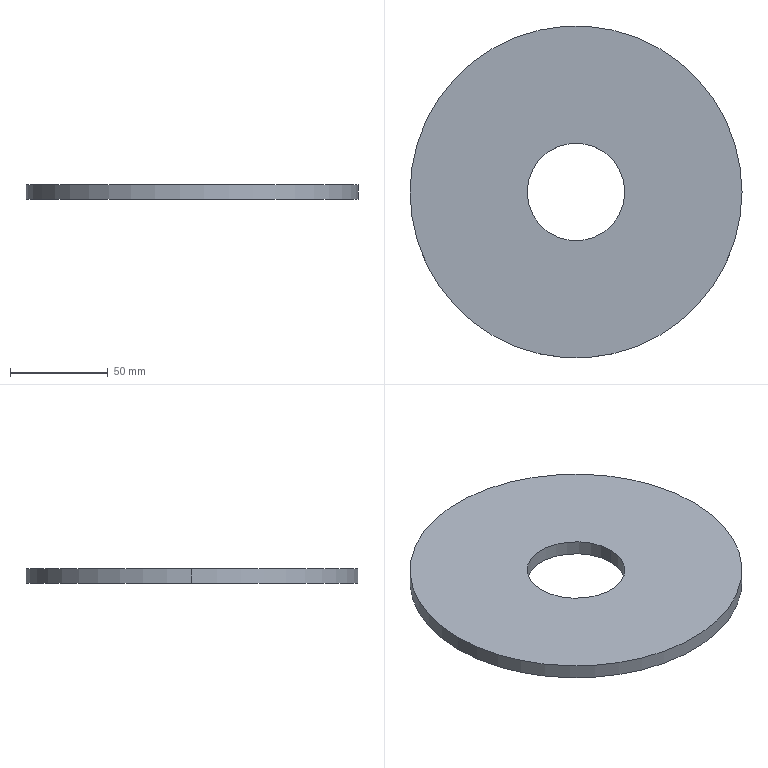Part | SolidWorks | features Cut 1, Extrusion 1 | 1 solid | 6 faces | box 170 x 170 x 7.5 mm | volume 155509 mm3 | cylinder 4 | plane 2 | commonest cylinder face diameters 50 x2 170 x2
STEP:
#1=CARTESIAN_POINT('',(-25.,0.,0.));
#2=VERTEX_POINT('',#1);
#3=CARTESIAN_POINT('',(25.,0.,0.));
#4=VERTEX_POINT('',#3);
#5=CARTESIAN_POINT('',(0.,0.,0.));
#6=DIRECTION('',(0.,0.,1.));
#7=DIRECTION('',(1.,0.,0.));
#8=AXIS2_PLACEMENT_3D('',#5,#6,#7);
#9=CIRCLE('',#8,25.);
#10=EDGE_CURVE('',#2,#4,#9,.T.);
#11=ORIENTED_EDGE('',*,*,#10,.F.);
#12=CARTESIAN_POINT('',(-25.,0.,7.5));
#13=VERTEX_POINT('',#12);
#14=CARTESIAN_POINT('',(-25.,0.,0.));
#15=DIRECTION('',(0.,0.,1.));
#16=VECTOR('',#15,1000.);
#17=LINE('',#14,#16);
#18=EDGE_CURVE('',#2,#13,#17,.T.);
#19=ORIENTED_EDGE('',*,*,#18,.T.);
#20=CARTESIAN_POINT('',(25.,0.,7.5));
#21=VERTEX_POINT('',#20);
#22=CARTESIAN_POINT('',(0.,0.,7.5));
#23=DIRECTION('',(0.,0.,1.));
#24=DIRECTION('',(1.,0.,0.));
#25=AXIS2_PLACEMENT_3D('',#22,#23,#24);
#26=CIRCLE('',#25,25.);
#27=EDGE_CURVE('',#13,#21,#26,.T.);
#28=ORIENTED_EDGE('',*,*,#27,.T.);
#29=CARTESIAN_POINT('',(25.,0.,0.));
#30=DIRECTION('',(0.,0.,1.));
#31=VECTOR('',#30,1000.);
#32=LINE('',#29,#31);
#33=EDGE_CURVE('',#4,#21,#32,.T.);
#34=ORIENTED_EDGE('',*,*,#33,.F.);
#35=EDGE_LOOP('',(#11,#19,#28,#34));
#36=FACE_OUTER_BOUND('',#35,.T.);
#37=CARTESIAN_POINT('',(0.,0.,0.));
#38=DIRECTION('',(0.,0.,1.));
#39=DIRECTION('',(1.,0.,0.));
#40=AXIS2_PLACEMENT_3D('',#37,#38,#39);
#41=CYLINDRICAL_SURFACE('',#40,25.);
#42=ADVANCED_FACE('',(#36),#41,.F.);
#43=CARTESIAN_POINT('',(85.,0.,7.5));
#44=VERTEX_POINT('',#43);
#45=CARTESIAN_POINT('',(-85.,0.,7.5));
#46=VERTEX_POINT('',#45);
#47=CARTESIAN_POINT('',(0.,0.,7.5));
#48=DIRECTION('',(0.,0.,1.));
#49=DIRECTION('',(1.,0.,0.));
#50=AXIS2_PLACEMENT_3D('',#47,#48,#49);
#51=CIRCLE('',#50,85.);
#52=EDGE_CURVE('',#44,#46,#51,.T.);
#53=ORIENTED_EDGE('',*,*,#52,.F.);
#54=CARTESIAN_POINT('',(85.,0.,0.));
#55=VERTEX_POINT('',#54);
#56=CARTESIAN_POINT('',(85.,0.,7.5));
#57=DIRECTION('',(0.,0.,-1.));
#58=VECTOR('',#57,1000.);
#59=LINE('',#56,#58);
#60=EDGE_CURVE('',#44,#55,#59,.T.);
#61=ORIENTED_EDGE('',*,*,#60,.T.);
#62=CARTESIAN_POINT('',(-85.,0.,0.));
#63=VERTEX_POINT('',#62);
#64=CARTESIAN_POINT('',(0.,0.,0.));
#65=DIRECTION('',(0.,0.,1.));
#66=DIRECTION('',(1.,0.,0.));
#67=AXIS2_PLACEMENT_3D('',#64,#65,#66);
#68=CIRCLE('',#67,85.);
#69=EDGE_CURVE('',#55,#63,#68,.T.);
#70=ORIENTED_EDGE('',*,*,#69,.T.);
#71=CARTESIAN_POINT('',(-85.,0.,7.5));
#72=DIRECTION('',(0.,0.,-1.));
#73=VECTOR('',#72,1000.);
#74=LINE('',#71,#73);
#75=EDGE_CURVE('',#46,#63,#74,.T.);
#76=ORIENTED_EDGE('',*,*,#75,.F.);
#77=EDGE_LOOP('',(#53,#61,#70,#76));
#78=FACE_OUTER_BOUND('',#77,.T.);
#79=CARTESIAN_POINT('',(0.,0.,7.5));
#80=DIRECTION('',(0.,0.,-1.));
#81=DIRECTION('',(-1.,0.,0.));
#82=AXIS2_PLACEMENT_3D('',#79,#80,#81);
#83=CYLINDRICAL_SURFACE('',#82,85.);
#84=ADVANCED_FACE('',(#78),#83,.T.);
#85=ORIENTED_EDGE('',*,*,#60,.F.);
#86=CARTESIAN_POINT('',(0.,0.,7.5));
#87=DIRECTION('',(0.,0.,1.));
#88=DIRECTION('',(1.,0.,0.));
#89=AXIS2_PLACEMENT_3D('',#86,#87,#88);
#90=CIRCLE('',#89,85.);
#91=EDGE_CURVE('',#46,#44,#90,.T.);
#92=ORIENTED_EDGE('',*,*,#91,.F.);
#93=ORIENTED_EDGE('',*,*,#75,.T.);
#94=CARTESIAN_POINT('',(0.,0.,0.));
#95=DIRECTION('',(0.,0.,1.));
#96=DIRECTION('',(1.,0.,0.));
#97=AXIS2_PLACEMENT_3D('',#94,#95,#96);
#98=CIRCLE('',#97,85.);
#99=EDGE_CURVE('',#63,#55,#98,.T.);
#100=ORIENTED_EDGE('',*,*,#99,.T.);
#101=EDGE_LOOP('',(#85,#92,#93,#100));
#102=FACE_OUTER_BOUND('',#101,.T.);
#103=CARTESIAN_POINT('',(0.,0.,7.5));
#104=DIRECTION('',(0.,0.,-1.));
#105=DIRECTION('',(-1.,0.,0.));
#106=AXIS2_PLACEMENT_3D('',#103,#104,#105);
#107=CYLINDRICAL_SURFACE('',#106,85.);
#108=ADVANCED_FACE('',(#102),#107,.T.);
#109=CARTESIAN_POINT('',(0.,0.,7.5));
#110=DIRECTION('',(0.,0.,1.));
#111=DIRECTION('',(1.,0.,0.));
#112=AXIS2_PLACEMENT_3D('',#109,#110,#111);
#113=CIRCLE('',#112,25.);
#114=EDGE_CURVE('',#21,#13,#113,.T.);
#115=ORIENTED_EDGE('',*,*,#114,.F.);
#116=ORIENTED_EDGE('',*,*,#27,.F.);
#117=EDGE_LOOP('',(#115,#116));
#118=FACE_BOUND('',#117,.T.);
#119=ORIENTED_EDGE('',*,*,#91,.T.);
#120=ORIENTED_EDGE('',*,*,#52,.T.);
#121=EDGE_LOOP('',(#119,#120));
#122=FACE_OUTER_BOUND('',#121,.T.);
#123=CARTESIAN_POINT('',(0.,0.,7.5));
#124=DIRECTION('',(0.,0.,1.));
#125=DIRECTION('',(1.,0.,0.));
#126=AXIS2_PLACEMENT_3D('',#123,#124,#125);
#127=PLANE('',#126);
#128=ADVANCED_FACE('',(#118,#122),#127,.T.);
#129=CARTESIAN_POINT('',(0.,0.,0.));
#130=DIRECTION('',(0.,0.,1.));
#131=DIRECTION('',(1.,0.,0.));
#132=AXIS2_PLACEMENT_3D('',#129,#130,#131);
#133=CIRCLE('',#132,25.);
#134=EDGE_CURVE('',#4,#2,#133,.T.);
#135=ORIENTED_EDGE('',*,*,#134,.T.);
#136=ORIENTED_EDGE('',*,*,#10,.T.);
#137=EDGE_LOOP('',(#135,#136));
#138=FACE_BOUND('',#137,.T.);
#139=ORIENTED_EDGE('',*,*,#99,.F.);
#140=ORIENTED_EDGE('',*,*,#69,.F.);
#141=EDGE_LOOP('',(#139,#140));
#142=FACE_OUTER_BOUND('',#141,.T.);
#143=CARTESIAN_POINT('',(0.,0.,0.));
#144=DIRECTION('',(0.,0.,1.));
#145=DIRECTION('',(1.,0.,0.));
#146=AXIS2_PLACEMENT_3D('',#143,#144,#145);
#147=PLANE('',#146);
#148=ADVANCED_FACE('',(#138,#142),#147,.F.);
#149=ORIENTED_EDGE('',*,*,#18,.F.);
#150=ORIENTED_EDGE('',*,*,#134,.F.);
#151=ORIENTED_EDGE('',*,*,#33,.T.);
#152=ORIENTED_EDGE('',*,*,#114,.T.);
#153=EDGE_LOOP('',(#149,#150,#151,#152));
#154=FACE_OUTER_BOUND('',#153,.T.);
#155=CARTESIAN_POINT('',(0.,0.,0.));
#156=DIRECTION('',(0.,0.,1.));
#157=DIRECTION('',(1.,0.,0.));
#158=AXIS2_PLACEMENT_3D('',#155,#156,#157);
#159=CYLINDRICAL_SURFACE('',#158,25.);
#160=ADVANCED_FACE('',(#154),#159,.F.);
#161=CLOSED_SHELL('',(#42,#84,#108,#128,#148,#160));
#162=MANIFOLD_SOLID_BREP('',#161);
#163=CARTESIAN_POINT('',(0.,0.,0.));
#164=DIRECTION('',(0.,0.,1.));
#165=DIRECTION('',(1.,0.,0.));
#166=AXIS2_PLACEMENT_3D('',#163,#164,#165);
#167=(LENGTH_UNIT()NAMED_UNIT(*)SI_UNIT(.MILLI.,.METRE.));
#168=UNCERTAINTY_MEASURE_WITH_UNIT(LENGTH_MEASURE(0.00001),#167,'','');
#169=(NAMED_UNIT(*)PLANE_ANGLE_UNIT()SI_UNIT($,.RADIAN.));
#170=(NAMED_UNIT(*)SI_UNIT($,.STERADIAN.)SOLID_ANGLE_UNIT());
#171=(GEOMETRIC_REPRESENTATION_CONTEXT(3)GLOBAL_UNCERTAINTY_ASSIGNED_CONTEXT((#168))GLOBAL_UNIT_ASSIGNED_CONTEXT((#167,#169,#170))REPRESENTATION_CONTEXT('',''));
#172=ADVANCED_BREP_SHAPE_REPRESENTATION('',(#162,#166),#171);